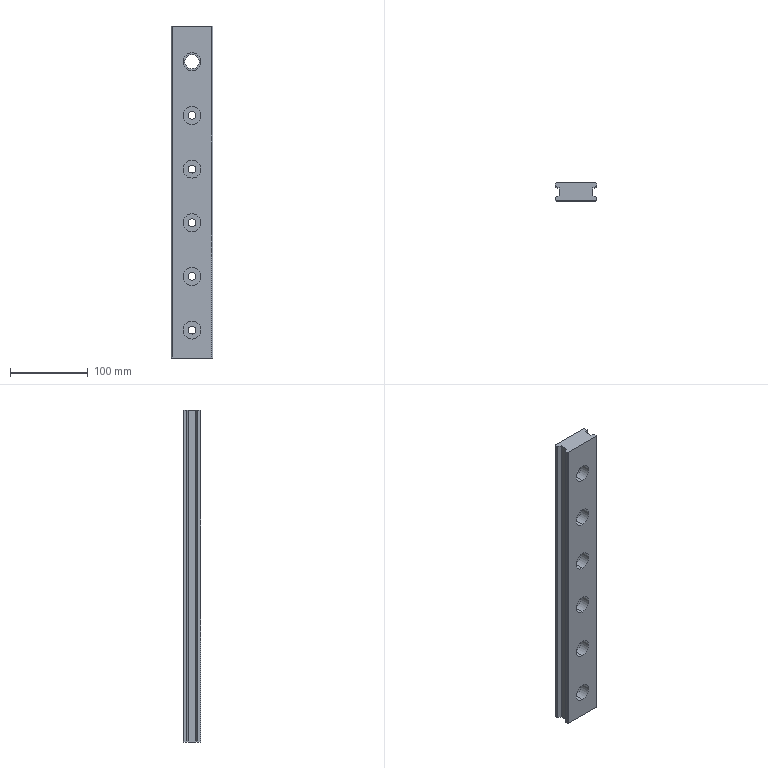Part | SolidWorks | features BaseBody 1 | 1 solid | 48 faces | box 53.538 x 23.077 x 428.351 mm | volume 438596 mm3 | cylinder 24 | plane 24 | commonest cylinder face diameters 23.077 x12 10.385 x10 18.462 x2
STEP:
#1=CARTESIAN_POINT('',(57.247,344.808,-35.962));
#2=VERTEX_POINT('',#1);
#3=CARTESIAN_POINT('',(57.247,344.808,-25.577));
#4=VERTEX_POINT('',#3);
#5=CARTESIAN_POINT('',(57.247,344.808,-30.769));
#6=DIRECTION('',(0.,1.,0.));
#7=DIRECTION('',(0.,0.,1.));
#8=AXIS2_PLACEMENT_3D('',#5,#6,#7);
#9=CIRCLE('',#8,5.192);
#10=EDGE_CURVE('',#2,#4,#9,.T.);
#11=ORIENTED_EDGE('',*,*,#10,.F.);
#12=CARTESIAN_POINT('',(57.247,354.5,-35.962));
#13=VERTEX_POINT('',#12);
#14=CARTESIAN_POINT('',(57.247,329.115,-35.962));
#15=DIRECTION('',(0.,1.,0.));
#16=VECTOR('',#15,1000.);
#17=LINE('',#14,#16);
#18=EDGE_CURVE('',#2,#13,#17,.T.);
#19=ORIENTED_EDGE('',*,*,#18,.T.);
#20=CARTESIAN_POINT('',(57.247,354.5,-25.577));
#21=VERTEX_POINT('',#20);
#22=CARTESIAN_POINT('',(57.247,354.5,-30.769));
#23=DIRECTION('',(0.,1.,0.));
#24=DIRECTION('',(0.,0.,1.));
#25=AXIS2_PLACEMENT_3D('',#22,#23,#24);
#26=CIRCLE('',#25,5.192);
#27=EDGE_CURVE('',#13,#21,#26,.T.);
#28=ORIENTED_EDGE('',*,*,#27,.T.);
#29=CARTESIAN_POINT('',(57.247,329.115,-25.577));
#30=DIRECTION('',(0.,1.,0.));
#31=VECTOR('',#30,1000.);
#32=LINE('',#29,#31);
#33=EDGE_CURVE('',#4,#21,#32,.T.);
#34=ORIENTED_EDGE('',*,*,#33,.F.);
#35=EDGE_LOOP('',(#11,#19,#28,#34));
#36=FACE_OUTER_BOUND('',#35,.T.);
#37=CARTESIAN_POINT('',(57.247,329.115,-30.769));
#38=DIRECTION('',(0.,1.,0.));
#39=DIRECTION('',(0.,0.,1.));
#40=AXIS2_PLACEMENT_3D('',#37,#38,#39);
#41=CYLINDRICAL_SURFACE('',#40,5.192);
#42=ADVANCED_FACE('',(#36),#41,.F.);
#43=CARTESIAN_POINT('',(57.247,344.808,102.5));
#44=VERTEX_POINT('',#43);
#45=CARTESIAN_POINT('',(57.247,344.808,112.885));
#46=VERTEX_POINT('',#45);
#47=CARTESIAN_POINT('',(57.247,344.808,107.692));
#48=DIRECTION('',(0.,1.,0.));
#49=DIRECTION('',(0.,0.,1.));
#50=AXIS2_PLACEMENT_3D('',#47,#48,#49);
#51=CIRCLE('',#50,5.192);
#52=EDGE_CURVE('',#44,#46,#51,.T.);
#53=ORIENTED_EDGE('',*,*,#52,.F.);
#54=CARTESIAN_POINT('',(57.247,354.5,102.5));
#55=VERTEX_POINT('',#54);
#56=CARTESIAN_POINT('',(57.247,329.115,102.5));
#57=DIRECTION('',(0.,1.,0.));
#58=VECTOR('',#57,1000.);
#59=LINE('',#56,#58);
#60=EDGE_CURVE('',#44,#55,#59,.T.);
#61=ORIENTED_EDGE('',*,*,#60,.T.);
#62=CARTESIAN_POINT('',(57.247,354.5,112.885));
#63=VERTEX_POINT('',#62);
#64=CARTESIAN_POINT('',(57.247,354.5,107.692));
#65=DIRECTION('',(0.,1.,0.));
#66=DIRECTION('',(0.,0.,1.));
#67=AXIS2_PLACEMENT_3D('',#64,#65,#66);
#68=CIRCLE('',#67,5.192);
#69=EDGE_CURVE('',#55,#63,#68,.T.);
#70=ORIENTED_EDGE('',*,*,#69,.T.);
#71=CARTESIAN_POINT('',(57.247,329.115,112.885));
#72=DIRECTION('',(0.,1.,0.));
#73=VECTOR('',#72,1000.);
#74=LINE('',#71,#73);
#75=EDGE_CURVE('',#46,#63,#74,.T.);
#76=ORIENTED_EDGE('',*,*,#75,.F.);
#77=EDGE_LOOP('',(#53,#61,#70,#76));
#78=FACE_OUTER_BOUND('',#77,.T.);
#79=CARTESIAN_POINT('',(57.247,329.115,107.692));
#80=DIRECTION('',(0.,1.,0.));
#81=DIRECTION('',(0.,0.,1.));
#82=AXIS2_PLACEMENT_3D('',#79,#80,#81);
#83=CYLINDRICAL_SURFACE('',#82,5.192);
#84=ADVANCED_FACE('',(#78),#83,.F.);
#85=CARTESIAN_POINT('',(57.247,344.808,236.923));
#86=VERTEX_POINT('',#85);
#87=CARTESIAN_POINT('',(57.247,344.808,255.385));
#88=VERTEX_POINT('',#87);
#89=CARTESIAN_POINT('',(57.247,344.808,246.154));
#90=DIRECTION('',(0.,1.,0.));
#91=DIRECTION('',(0.,0.,1.));
#92=AXIS2_PLACEMENT_3D('',#89,#90,#91);
#93=CIRCLE('',#92,9.231);
#94=EDGE_CURVE('',#86,#88,#93,.T.);
#95=ORIENTED_EDGE('',*,*,#94,.F.);
#96=CARTESIAN_POINT('',(57.247,354.5,236.923));
#97=VERTEX_POINT('',#96);
#98=CARTESIAN_POINT('',(57.247,329.115,236.923));
#99=DIRECTION('',(0.,1.,0.));
#100=VECTOR('',#99,1000.);
#101=LINE('',#98,#100);
#102=EDGE_CURVE('',#86,#97,#101,.T.);
#103=ORIENTED_EDGE('',*,*,#102,.T.);
#104=CARTESIAN_POINT('',(57.247,354.5,255.385));
#105=VERTEX_POINT('',#104);
#106=CARTESIAN_POINT('',(57.247,354.5,246.154));
#107=DIRECTION('',(0.,1.,0.));
#108=DIRECTION('',(0.,0.,1.));
#109=AXIS2_PLACEMENT_3D('',#106,#107,#108);
#110=CIRCLE('',#109,9.231);
#111=EDGE_CURVE('',#97,#105,#110,.T.);
#112=ORIENTED_EDGE('',*,*,#111,.T.);
#113=CARTESIAN_POINT('',(57.247,329.115,255.385));
#114=DIRECTION('',(0.,1.,0.));
#115=VECTOR('',#114,1000.);
#116=LINE('',#113,#115);
#117=EDGE_CURVE('',#88,#105,#116,.T.);
#118=ORIENTED_EDGE('',*,*,#117,.F.);
#119=EDGE_LOOP('',(#95,#103,#112,#118));
#120=FACE_OUTER_BOUND('',#119,.T.);
#121=CARTESIAN_POINT('',(57.247,329.115,246.154));
#122=DIRECTION('',(0.,1.,0.));
#123=DIRECTION('',(0.,0.,1.));
#124=AXIS2_PLACEMENT_3D('',#121,#122,#123);
#125=CYLINDRICAL_SURFACE('',#124,9.231);
#126=ADVANCED_FACE('',(#120),#125,.F.);
#127=CARTESIAN_POINT('',(57.247,344.808,-105.192));
#128=VERTEX_POINT('',#127);
#129=CARTESIAN_POINT('',(57.247,344.808,-94.808));
#130=VERTEX_POINT('',#129);
#131=CARTESIAN_POINT('',(57.247,344.808,-100.));
#132=DIRECTION('',(0.,1.,0.));
#133=DIRECTION('',(0.,0.,1.));
#134=AXIS2_PLACEMENT_3D('',#131,#132,#133);
#135=CIRCLE('',#134,5.192);
#136=EDGE_CURVE('',#128,#130,#135,.T.);
#137=ORIENTED_EDGE('',*,*,#136,.F.);
#138=CARTESIAN_POINT('',(57.247,354.5,-105.192));
#139=VERTEX_POINT('',#138);
#140=CARTESIAN_POINT('',(57.247,329.115,-105.192));
#141=DIRECTION('',(0.,1.,0.));
#142=VECTOR('',#141,1000.);
#143=LINE('',#140,#142);
#144=EDGE_CURVE('',#128,#139,#143,.T.);
#145=ORIENTED_EDGE('',*,*,#144,.T.);
#146=CARTESIAN_POINT('',(57.247,354.5,-94.808));
#147=VERTEX_POINT('',#146);
#148=CARTESIAN_POINT('',(57.247,354.5,-100.));
#149=DIRECTION('',(0.,1.,0.));
#150=DIRECTION('',(0.,0.,1.));
#151=AXIS2_PLACEMENT_3D('',#148,#149,#150);
#152=CIRCLE('',#151,5.192);
#153=EDGE_CURVE('',#139,#147,#152,.T.);
#154=ORIENTED_EDGE('',*,*,#153,.T.);
#155=CARTESIAN_POINT('',(57.247,329.115,-94.808));
#156=DIRECTION('',(0.,1.,0.));
#157=VECTOR('',#156,1000.);
#158=LINE('',#155,#157);
#159=EDGE_CURVE('',#130,#147,#158,.T.);
#160=ORIENTED_EDGE('',*,*,#159,.F.);
#161=EDGE_LOOP('',(#137,#145,#154,#160));
#162=FACE_OUTER_BOUND('',#161,.T.);
#163=CARTESIAN_POINT('',(57.247,329.115,-100.));
#164=DIRECTION('',(0.,1.,0.));
#165=DIRECTION('',(0.,0.,1.));
#166=AXIS2_PLACEMENT_3D('',#163,#164,#165);
#167=CYLINDRICAL_SURFACE('',#166,5.192);
#168=ADVANCED_FACE('',(#162),#167,.F.);
#169=CARTESIAN_POINT('',(57.247,344.808,171.731));
#170=VERTEX_POINT('',#169);
#171=CARTESIAN_POINT('',(57.247,344.808,182.115));
#172=VERTEX_POINT('',#171);
#173=CARTESIAN_POINT('',(57.247,344.808,176.923));
#174=DIRECTION('',(0.,1.,0.));
#175=DIRECTION('',(0.,0.,1.));
#176=AXIS2_PLACEMENT_3D('',#173,#174,#175);
#177=CIRCLE('',#176,5.192);
#178=EDGE_CURVE('',#170,#172,#177,.T.);
#179=ORIENTED_EDGE('',*,*,#178,.F.);
#180=CARTESIAN_POINT('',(57.247,354.5,171.731));
#181=VERTEX_POINT('',#180);
#182=CARTESIAN_POINT('',(57.247,329.115,171.731));
#183=DIRECTION('',(0.,1.,0.));
#184=VECTOR('',#183,1000.);
#185=LINE('',#182,#184);
#186=EDGE_CURVE('',#170,#181,#185,.T.);
#187=ORIENTED_EDGE('',*,*,#186,.T.);
#188=CARTESIAN_POINT('',(57.247,354.5,182.115));
#189=VERTEX_POINT('',#188);
#190=CARTESIAN_POINT('',(57.247,354.5,176.923));
#191=DIRECTION('',(0.,1.,0.));
#192=DIRECTION('',(0.,0.,1.));
#193=AXIS2_PLACEMENT_3D('',#190,#191,#192);
#194=CIRCLE('',#193,5.192);
#195=EDGE_CURVE('',#181,#189,#194,.T.);
#196=ORIENTED_EDGE('',*,*,#195,.T.);
#197=CARTESIAN_POINT('',(57.247,329.115,182.115));
#198=DIRECTION('',(0.,1.,0.));
#199=VECTOR('',#198,1000.);
#200=LINE('',#197,#199);
#201=EDGE_CURVE('',#172,#189,#200,.T.);
#202=ORIENTED_EDGE('',*,*,#201,.F.);
#203=EDGE_LOOP('',(#179,#187,#196,#202));
#204=FACE_OUTER_BOUND('',#203,.T.);
#205=CARTESIAN_POINT('',(57.247,329.115,176.923));
#206=DIRECTION('',(0.,1.,0.));
#207=DIRECTION('',(0.,0.,1.));
#208=AXIS2_PLACEMENT_3D('',#205,#206,#207);
#209=CYLINDRICAL_SURFACE('',#208,5.192);
#210=ADVANCED_FACE('',(#204),#209,.F.);
#211=CARTESIAN_POINT('',(57.247,344.808,33.269));
#212=VERTEX_POINT('',#211);
#213=CARTESIAN_POINT('',(57.247,344.808,43.654));
#214=VERTEX_POINT('',#213);
#215=CARTESIAN_POINT('',(57.247,344.808,38.462));
#216=DIRECTION('',(0.,1.,0.));
#217=DIRECTION('',(0.,0.,1.));
#218=AXIS2_PLACEMENT_3D('',#215,#216,#217);
#219=CIRCLE('',#218,5.192);
#220=EDGE_CURVE('',#212,#214,#219,.T.);
#221=ORIENTED_EDGE('',*,*,#220,.F.);
#222=CARTESIAN_POINT('',(57.247,354.5,33.269));
#223=VERTEX_POINT('',#222);
#224=CARTESIAN_POINT('',(57.247,329.115,33.269));
#225=DIRECTION('',(0.,1.,0.));
#226=VECTOR('',#225,1000.);
#227=LINE('',#224,#226);
#228=EDGE_CURVE('',#212,#223,#227,.T.);
#229=ORIENTED_EDGE('',*,*,#228,.T.);
#230=CARTESIAN_POINT('',(57.247,354.5,43.654));
#231=VERTEX_POINT('',#230);
#232=CARTESIAN_POINT('',(57.247,354.5,38.462));
#233=DIRECTION('',(0.,1.,0.));
#234=DIRECTION('',(0.,0.,1.));
#235=AXIS2_PLACEMENT_3D('',#232,#233,#234);
#236=CIRCLE('',#235,5.192);
#237=EDGE_CURVE('',#223,#231,#236,.T.);
#238=ORIENTED_EDGE('',*,*,#237,.T.);
#239=CARTESIAN_POINT('',(57.247,329.115,43.654));
#240=DIRECTION('',(0.,1.,0.));
#241=VECTOR('',#240,1000.);
#242=LINE('',#239,#241);
#243=EDGE_CURVE('',#214,#231,#242,.T.);
#244=ORIENTED_EDGE('',*,*,#243,.F.);
#245=EDGE_LOOP('',(#221,#229,#238,#244));
#246=FACE_OUTER_BOUND('',#245,.T.);
#247=CARTESIAN_POINT('',(57.247,329.115,38.462));
#248=DIRECTION('',(0.,1.,0.));
#249=DIRECTION('',(0.,0.,1.));
#250=AXIS2_PLACEMENT_3D('',#247,#248,#249);
#251=CYLINDRICAL_SURFACE('',#250,5.192);
#252=ADVANCED_FACE('',(#246),#251,.F.);
#253=CARTESIAN_POINT('',(57.247,331.423,-19.231));
#254=VERTEX_POINT('',#253);
#255=CARTESIAN_POINT('',(57.247,331.423,-42.308));
#256=VERTEX_POINT('',#255);
#257=CARTESIAN_POINT('',(57.247,331.423,-30.769));
#258=DIRECTION('',(0.,-1.,0.));
#259=DIRECTION('',(0.,0.,1.));
#260=AXIS2_PLACEMENT_3D('',#257,#258,#259);
#261=CIRCLE('',#260,11.538);
#262=EDGE_CURVE('',#254,#256,#261,.T.);
#263=ORIENTED_EDGE('',*,*,#262,.T.);
#264=CARTESIAN_POINT('',(57.247,344.808,-42.308));
#265=VERTEX_POINT('',#264);
#266=CARTESIAN_POINT('',(57.247,329.115,-42.308));
#267=DIRECTION('',(0.,1.,0.));
#268=VECTOR('',#267,1000.);
#269=LINE('',#266,#268);
#270=EDGE_CURVE('',#256,#265,#269,.T.);
#271=ORIENTED_EDGE('',*,*,#270,.T.);
#272=CARTESIAN_POINT('',(57.247,344.808,-19.231));
#273=VERTEX_POINT('',#272);
#274=CARTESIAN_POINT('',(57.247,344.808,-30.769));
#275=DIRECTION('',(0.,-1.,0.));
#276=DIRECTION('',(0.,0.,1.));
#277=AXIS2_PLACEMENT_3D('',#274,#275,#276);
#278=CIRCLE('',#277,11.538);
#279=EDGE_CURVE('',#273,#265,#278,.T.);
#280=ORIENTED_EDGE('',*,*,#279,.F.);
#281=CARTESIAN_POINT('',(57.247,329.115,-19.231));
#282=DIRECTION('',(0.,1.,0.));
#283=VECTOR('',#282,1000.);
#284=LINE('',#281,#283);
#285=EDGE_CURVE('',#254,#273,#284,.T.);
#286=ORIENTED_EDGE('',*,*,#285,.F.);
#287=EDGE_LOOP('',(#263,#271,#280,#286));
#288=FACE_OUTER_BOUND('',#287,.T.);
#289=CARTESIAN_POINT('',(57.247,329.115,-30.769));
#290=DIRECTION('',(0.,1.,0.));
#291=DIRECTION('',(0.,0.,1.));
#292=AXIS2_PLACEMENT_3D('',#289,#290,#291);
#293=CYLINDRICAL_SURFACE('',#292,11.538);
#294=ADVANCED_FACE('',(#288),#293,.F.);
#295=CARTESIAN_POINT('',(57.247,331.423,119.231));
#296=VERTEX_POINT('',#295);
#297=CARTESIAN_POINT('',(57.247,331.423,96.154));
#298=VERTEX_POINT('',#297);
#299=CARTESIAN_POINT('',(57.247,331.423,107.692));
#300=DIRECTION('',(0.,-1.,0.));
#301=DIRECTION('',(0.,0.,1.));
#302=AXIS2_PLACEMENT_3D('',#299,#300,#301);
#303=CIRCLE('',#302,11.538);
#304=EDGE_CURVE('',#296,#298,#303,.T.);
#305=ORIENTED_EDGE('',*,*,#304,.T.);
#306=CARTESIAN_POINT('',(57.247,344.808,96.154));
#307=VERTEX_POINT('',#306);
#308=CARTESIAN_POINT('',(57.247,329.115,96.154));
#309=DIRECTION('',(0.,1.,0.));
#310=VECTOR('',#309,1000.);
#311=LINE('',#308,#310);
#312=EDGE_CURVE('',#298,#307,#311,.T.);
#313=ORIENTED_EDGE('',*,*,#312,.T.);
#314=CARTESIAN_POINT('',(57.247,344.808,119.231));
#315=VERTEX_POINT('',#314);
#316=CARTESIAN_POINT('',(57.247,344.808,107.692));
#317=DIRECTION('',(0.,-1.,0.));
#318=DIRECTION('',(0.,0.,1.));
#319=AXIS2_PLACEMENT_3D('',#316,#317,#318);
#320=CIRCLE('',#319,11.538);
#321=EDGE_CURVE('',#315,#307,#320,.T.);
#322=ORIENTED_EDGE('',*,*,#321,.F.);
#323=CARTESIAN_POINT('',(57.247,329.115,119.231));
#324=DIRECTION('',(0.,1.,0.));
#325=VECTOR('',#324,1000.);
#326=LINE('',#323,#325);
#327=EDGE_CURVE('',#296,#315,#326,.T.);
#328=ORIENTED_EDGE('',*,*,#327,.F.);
#329=EDGE_LOOP('',(#305,#313,#322,#328));
#330=FACE_OUTER_BOUND('',#329,.T.);
#331=CARTESIAN_POINT('',(57.247,329.115,107.692));
#332=DIRECTION('',(0.,1.,0.));
#333=DIRECTION('',(0.,0.,1.));
#334=AXIS2_PLACEMENT_3D('',#331,#332,#333);
#335=CYLINDRICAL_SURFACE('',#334,11.538);
#336=ADVANCED_FACE('',(#330),#335,.F.);
#337=CARTESIAN_POINT('',(57.247,331.423,257.692));
#338=VERTEX_POINT('',#337);
#339=CARTESIAN_POINT('',(57.247,331.423,234.615));
#340=VERTEX_POINT('',#339);
#341=CARTESIAN_POINT('',(57.247,331.423,246.154));
#342=DIRECTION('',(0.,-1.,0.));
#343=DIRECTION('',(0.,0.,1.));
#344=AXIS2_PLACEMENT_3D('',#341,#342,#343);
#345=CIRCLE('',#344,11.538);
#346=EDGE_CURVE('',#338,#340,#345,.T.);
#347=ORIENTED_EDGE('',*,*,#346,.T.);
#348=CARTESIAN_POINT('',(57.247,344.808,234.615));
#349=VERTEX_POINT('',#348);
#350=CARTESIAN_POINT('',(57.247,329.115,234.615));
#351=DIRECTION('',(0.,1.,0.));
#352=VECTOR('',#351,1000.);
#353=LINE('',#350,#352);
#354=EDGE_CURVE('',#340,#349,#353,.T.);
#355=ORIENTED_EDGE('',*,*,#354,.T.);
#356=CARTESIAN_POINT('',(57.247,344.808,257.692));
#357=VERTEX_POINT('',#356);
#358=CARTESIAN_POINT('',(57.247,344.808,246.154));
#359=DIRECTION('',(0.,-1.,0.));
#360=DIRECTION('',(0.,0.,1.));
#361=AXIS2_PLACEMENT_3D('',#358,#359,#360);
#362=CIRCLE('',#361,11.538);
#363=EDGE_CURVE('',#357,#349,#362,.T.);
#364=ORIENTED_EDGE('',*,*,#363,.F.);
#365=CARTESIAN_POINT('',(57.247,329.115,257.692));
#366=DIRECTION('',(0.,1.,0.));
#367=VECTOR('',#366,1000.);
#368=LINE('',#365,#367);
#369=EDGE_CURVE('',#338,#357,#368,.T.);
#370=ORIENTED_EDGE('',*,*,#369,.F.);
#371=EDGE_LOOP('',(#347,#355,#364,#370));
#372=FACE_OUTER_BOUND('',#371,.T.);
#373=CARTESIAN_POINT('',(57.247,329.115,246.154));
#374=DIRECTION('',(0.,1.,0.));
#375=DIRECTION('',(0.,0.,1.));
#376=AXIS2_PLACEMENT_3D('',#373,#374,#375);
#377=CYLINDRICAL_SURFACE('',#376,11.538);
#378=ADVANCED_FACE('',(#372),#377,.F.);
#379=CARTESIAN_POINT('',(57.247,331.423,-88.462));
#380=VERTEX_POINT('',#379);
#381=CARTESIAN_POINT('',(57.247,331.423,-111.538));
#382=VERTEX_POINT('',#381);
#383=CARTESIAN_POINT('',(57.247,331.423,-100.));
#384=DIRECTION('',(0.,-1.,0.));
#385=DIRECTION('',(0.,0.,1.));
#386=AXIS2_PLACEMENT_3D('',#383,#384,#385);
#387=CIRCLE('',#386,11.538);
#388=EDGE_CURVE('',#380,#382,#387,.T.);
#389=ORIENTED_EDGE('',*,*,#388,.T.);
#390=CARTESIAN_POINT('',(57.247,344.808,-111.538));
#391=VERTEX_POINT('',#390);
#392=CARTESIAN_POINT('',(57.247,329.115,-111.538));
#393=DIRECTION('',(0.,1.,0.));
#394=VECTOR('',#393,1000.);
#395=LINE('',#392,#394);
#396=EDGE_CURVE('',#382,#391,#395,.T.);
#397=ORIENTED_EDGE('',*,*,#396,.T.);
#398=CARTESIAN_POINT('',(57.247,344.808,-88.462));
#399=VERTEX_POINT('',#398);
#400=CARTESIAN_POINT('',(57.247,344.808,-100.));
#401=DIRECTION('',(0.,-1.,0.));
#402=DIRECTION('',(0.,0.,1.));
#403=AXIS2_PLACEMENT_3D('',#400,#401,#402);
#404=CIRCLE('',#403,11.538);
#405=EDGE_CURVE('',#399,#391,#404,.T.);
#406=ORIENTED_EDGE('',*,*,#405,.F.);
#407=CARTESIAN_POINT('',(57.247,329.115,-88.462));
#408=DIRECTION('',(0.,1.,0.));
#409=VECTOR('',#408,1000.);
#410=LINE('',#407,#409);
#411=EDGE_CURVE('',#380,#399,#410,.T.);
#412=ORIENTED_EDGE('',*,*,#411,.F.);
#413=EDGE_LOOP('',(#389,#397,#406,#412));
#414=FACE_OUTER_BOUND('',#413,.T.);
#415=CARTESIAN_POINT('',(57.247,329.115,-100.));
#416=DIRECTION('',(0.,1.,0.));
#417=DIRECTION('',(0.,0.,1.));
#418=AXIS2_PLACEMENT_3D('',#415,#416,#417);
#419=CYLINDRICAL_SURFACE('',#418,11.538);
#420=ADVANCED_FACE('',(#414),#419,.F.);
#421=CARTESIAN_POINT('',(57.247,331.423,188.462));
#422=VERTEX_POINT('',#421);
#423=CARTESIAN_POINT('',(57.247,331.423,165.385));
#424=VERTEX_POINT('',#423);
#425=CARTESIAN_POINT('',(57.247,331.423,176.923));
#426=DIRECTION('',(0.,-1.,0.));
#427=DIRECTION('',(0.,0.,1.));
#428=AXIS2_PLACEMENT_3D('',#425,#426,#427);
#429=CIRCLE('',#428,11.538);
#430=EDGE_CURVE('',#422,#424,#429,.T.);
#431=ORIENTED_EDGE('',*,*,#430,.T.);
#432=CARTESIAN_POINT('',(57.247,344.808,165.385));
#433=VERTEX_POINT('',#432);
#434=CARTESIAN_POINT('',(57.247,329.115,165.385));
#435=DIRECTION('',(0.,1.,0.));
#436=VECTOR('',#435,1000.);
#437=LINE('',#434,#436);
#438=EDGE_CURVE('',#424,#433,#437,.T.);
#439=ORIENTED_EDGE('',*,*,#438,.T.);
#440=CARTESIAN_POINT('',(57.247,344.808,188.462));
#441=VERTEX_POINT('',#440);
#442=CARTESIAN_POINT('',(57.247,344.808,176.923));
#443=DIRECTION('',(0.,-1.,0.));
#444=DIRECTION('',(0.,0.,1.));
#445=AXIS2_PLACEMENT_3D('',#442,#443,#444);
#446=CIRCLE('',#445,11.538);
#447=EDGE_CURVE('',#441,#433,#446,.T.);
#448=ORIENTED_EDGE('',*,*,#447,.F.);
#449=CARTESIAN_POINT('',(57.247,329.115,188.462));
#450=DIRECTION('',(0.,1.,0.));
#451=VECTOR('',#450,1000.);
#452=LINE('',#449,#451);
#453=EDGE_CURVE('',#422,#441,#452,.T.);
#454=ORIENTED_EDGE('',*,*,#453,.F.);
#455=EDGE_LOOP('',(#431,#439,#448,#454));
#456=FACE_OUTER_BOUND('',#455,.T.);
#457=CARTESIAN_POINT('',(57.247,329.115,176.923));
#458=DIRECTION('',(0.,1.,0.));
#459=DIRECTION('',(0.,0.,1.));
#460=AXIS2_PLACEMENT_3D('',#457,#458,#459);
#461=CYLINDRICAL_SURFACE('',#460,11.538);
#462=ADVANCED_FACE('',(#456),#461,.F.);
#463=CARTESIAN_POINT('',(57.247,331.423,50.));
#464=VERTEX_POINT('',#463);
#465=CARTESIAN_POINT('',(57.247,331.423,26.923));
#466=VERTEX_POINT('',#465);
#467=CARTESIAN_POINT('',(57.247,331.423,38.462));
#468=DIRECTION('',(0.,-1.,0.));
#469=DIRECTION('',(0.,0.,1.));
#470=AXIS2_PLACEMENT_3D('',#467,#468,#469);
#471=CIRCLE('',#470,11.538);
#472=EDGE_CURVE('',#464,#466,#471,.T.);
#473=ORIENTED_EDGE('',*,*,#472,.T.);
#474=CARTESIAN_POINT('',(57.247,344.808,26.923));
#475=VERTEX_POINT('',#474);
#476=CARTESIAN_POINT('',(57.247,329.115,26.923));
#477=DIRECTION('',(0.,1.,0.));
#478=VECTOR('',#477,1000.);
#479=LINE('',#476,#478);
#480=EDGE_CURVE('',#466,#475,#479,.T.);
#481=ORIENTED_EDGE('',*,*,#480,.T.);
#482=CARTESIAN_POINT('',(57.247,344.808,50.));
#483=VERTEX_POINT('',#482);
#484=CARTESIAN_POINT('',(57.247,344.808,38.462));
#485=DIRECTION('',(0.,-1.,0.));
#486=DIRECTION('',(0.,0.,1.));
#487=AXIS2_PLACEMENT_3D('',#484,#485,#486);
#488=CIRCLE('',#487,11.538);
#489=EDGE_CURVE('',#483,#475,#488,.T.);
#490=ORIENTED_EDGE('',*,*,#489,.F.);
#491=CARTESIAN_POINT('',(57.247,329.115,50.));
#492=DIRECTION('',(0.,1.,0.));
#493=VECTOR('',#492,1000.);
#494=LINE('',#491,#493);
#495=EDGE_CURVE('',#464,#483,#494,.T.);
#496=ORIENTED_EDGE('',*,*,#495,.F.);
#497=EDGE_LOOP('',(#473,#481,#490,#496));
#498=FACE_OUTER_BOUND('',#497,.T.);
#499=CARTESIAN_POINT('',(57.247,329.115,38.462));
#500=DIRECTION('',(0.,1.,0.));
#501=DIRECTION('',(0.,0.,1.));
#502=AXIS2_PLACEMENT_3D('',#499,#500,#501);
#503=CYLINDRICAL_SURFACE('',#502,11.538);
#504=ADVANCED_FACE('',(#498),#503,.F.);
#505=CARTESIAN_POINT('',(57.247,354.5,-30.769));
#506=DIRECTION('',(0.,1.,0.));
#507=DIRECTION('',(0.,0.,1.));
#508=AXIS2_PLACEMENT_3D('',#505,#506,#507);
#509=CIRCLE('',#508,5.192);
#510=EDGE_CURVE('',#21,#13,#509,.T.);
#511=ORIENTED_EDGE('',*,*,#510,.F.);
#512=ORIENTED_EDGE('',*,*,#27,.F.);
#513=EDGE_LOOP('',(#511,#512));
#514=FACE_BOUND('',#513,.T.);
#515=CARTESIAN_POINT('',(57.247,354.5,107.692));
#516=DIRECTION('',(0.,1.,0.));
#517=DIRECTION('',(0.,0.,1.));
#518=AXIS2_PLACEMENT_3D('',#515,#516,#517);
#519=CIRCLE('',#518,5.192);
#520=EDGE_CURVE('',#63,#55,#519,.T.);
#521=ORIENTED_EDGE('',*,*,#520,.F.);
#522=ORIENTED_EDGE('',*,*,#69,.F.);
#523=EDGE_LOOP('',(#521,#522));
#524=FACE_BOUND('',#523,.T.);
#525=CARTESIAN_POINT('',(57.247,354.5,246.154));
#526=DIRECTION('',(0.,1.,0.));
#527=DIRECTION('',(0.,0.,1.));
#528=AXIS2_PLACEMENT_3D('',#525,#526,#527);
#529=CIRCLE('',#528,9.231);
#530=EDGE_CURVE('',#105,#97,#529,.T.);
#531=ORIENTED_EDGE('',*,*,#530,.F.);
#532=ORIENTED_EDGE('',*,*,#111,.F.);
#533=EDGE_LOOP('',(#531,#532));
#534=FACE_BOUND('',#533,.T.);
#535=CARTESIAN_POINT('',(57.247,354.5,-100.));
#536=DIRECTION('',(0.,1.,0.));
#537=DIRECTION('',(0.,0.,1.));
#538=AXIS2_PLACEMENT_3D('',#535,#536,#537);
#539=CIRCLE('',#538,5.192);
#540=EDGE_CURVE('',#147,#139,#539,.T.);
#541=ORIENTED_EDGE('',*,*,#540,.F.);
#542=ORIENTED_EDGE('',*,*,#153,.F.);
#543=EDGE_LOOP('',(#541,#542));
#544=FACE_BOUND('',#543,.T.);
#545=CARTESIAN_POINT('',(57.247,354.5,176.923));
#546=DIRECTION('',(0.,1.,0.));
#547=DIRECTION('',(0.,0.,1.));
#548=AXIS2_PLACEMENT_3D('',#545,#546,#547);
#549=CIRCLE('',#548,5.192);
#550=EDGE_CURVE('',#189,#181,#549,.T.);
#551=ORIENTED_EDGE('',*,*,#550,.F.);
#552=ORIENTED_EDGE('',*,*,#195,.F.);
#553=EDGE_LOOP('',(#551,#552));
#554=FACE_BOUND('',#553,.T.);
#555=CARTESIAN_POINT('',(57.247,354.5,38.462));
#556=DIRECTION('',(0.,1.,0.));
#557=DIRECTION('',(0.,0.,1.));
#558=AXIS2_PLACEMENT_3D('',#555,#556,#557);
#559=CIRCLE('',#558,5.192);
#560=EDGE_CURVE('',#231,#223,#559,.T.);
#561=ORIENTED_EDGE('',*,*,#560,.F.);
#562=ORIENTED_EDGE('',*,*,#237,.F.);
#563=EDGE_LOOP('',(#561,#562));
#564=FACE_BOUND('',#563,.T.);
#565=CARTESIAN_POINT('',(31.631,354.5,292.308));
#566=VERTEX_POINT('',#565);
#567=CARTESIAN_POINT('',(31.631,354.5,-136.043));
#568=VERTEX_POINT('',#567);
#569=CARTESIAN_POINT('',(31.631,354.5,-284.615));
#570=DIRECTION('',(0.,0.,-1.));
#571=VECTOR('',#570,1000.);
#572=LINE('',#569,#571);
#573=EDGE_CURVE('',#566,#568,#572,.T.);
#574=ORIENTED_EDGE('',*,*,#573,.F.);
#575=CARTESIAN_POINT('',(82.862,354.5,292.308));
#576=VERTEX_POINT('',#575);
#577=CARTESIAN_POINT('',(31.631,354.5,292.308));
#578=DIRECTION('',(-1.,0.,0.));
#579=VECTOR('',#578,1000.);
#580=LINE('',#577,#579);
#581=EDGE_CURVE('',#576,#566,#580,.T.);
#582=ORIENTED_EDGE('',*,*,#581,.F.);
#583=CARTESIAN_POINT('',(82.862,354.5,-136.043));
#584=VERTEX_POINT('',#583);
#585=CARTESIAN_POINT('',(82.862,354.5,-284.615));
#586=DIRECTION('',(0.,0.,1.));
#587=VECTOR('',#586,1000.);
#588=LINE('',#585,#587);
#589=EDGE_CURVE('',#584,#576,#588,.T.);
#590=ORIENTED_EDGE('',*,*,#589,.F.);
#591=CARTESIAN_POINT('',(31.631,354.5,-136.043));
#592=DIRECTION('',(1.,0.,0.));
#593=VECTOR('',#592,1000.);
#594=LINE('',#591,#593);
#595=EDGE_CURVE('',#568,#584,#594,.T.);
#596=ORIENTED_EDGE('',*,*,#595,.F.);
#597=EDGE_LOOP('',(#574,#582,#590,#596));
#598=FACE_OUTER_BOUND('',#597,.T.);
#599=CARTESIAN_POINT('',(31.631,354.5,-284.615));
#600=DIRECTION('',(0.,-1.,0.));
#601=DIRECTION('',(0.,0.,-1.));
#602=AXIS2_PLACEMENT_3D('',#599,#600,#601);
#603=PLANE('',#602);
#604=ADVANCED_FACE('',(#514,#524,#534,#544,#554,#564,#598),#603,.F.);
#605=ORIENTED_EDGE('',*,*,#18,.F.);
#606=CARTESIAN_POINT('',(57.247,344.808,-30.769));
#607=DIRECTION('',(0.,1.,0.));
#608=DIRECTION('',(0.,0.,1.));
#609=AXIS2_PLACEMENT_3D('',#606,#607,#608);
#610=CIRCLE('',#609,5.192);
#611=EDGE_CURVE('',#4,#2,#610,.T.);
#612=ORIENTED_EDGE('',*,*,#611,.F.);
#613=ORIENTED_EDGE('',*,*,#33,.T.);
#614=ORIENTED_EDGE('',*,*,#510,.T.);
#615=EDGE_LOOP('',(#605,#612,#613,#614));
#616=FACE_OUTER_BOUND('',#615,.T.);
#617=CARTESIAN_POINT('',(57.247,329.115,-30.769));
#618=DIRECTION('',(0.,1.,0.));
#619=DIRECTION('',(0.,0.,1.));
#620=AXIS2_PLACEMENT_3D('',#617,#618,#619);
#621=CYLINDRICAL_SURFACE('',#620,5.192);
#622=ADVANCED_FACE('',(#616),#621,.F.);
#623=ORIENTED_EDGE('',*,*,#60,.F.);
#624=CARTESIAN_POINT('',(57.247,344.808,107.692));
#625=DIRECTION('',(0.,1.,0.));
#626=DIRECTION('',(0.,0.,1.));
#627=AXIS2_PLACEMENT_3D('',#624,#625,#626);
#628=CIRCLE('',#627,5.192);
#629=EDGE_CURVE('',#46,#44,#628,.T.);
#630=ORIENTED_EDGE('',*,*,#629,.F.);
#631=ORIENTED_EDGE('',*,*,#75,.T.);
#632=ORIENTED_EDGE('',*,*,#520,.T.);
#633=EDGE_LOOP('',(#623,#630,#631,#632));
#634=FACE_OUTER_BOUND('',#633,.T.);
#635=CARTESIAN_POINT('',(57.247,329.115,107.692));
#636=DIRECTION('',(0.,1.,0.));
#637=DIRECTION('',(0.,0.,1.));
#638=AXIS2_PLACEMENT_3D('',#635,#636,#637);
#639=CYLINDRICAL_SURFACE('',#638,5.192);
#640=ADVANCED_FACE('',(#634),#639,.F.);
#641=ORIENTED_EDGE('',*,*,#102,.F.);
#642=CARTESIAN_POINT('',(57.247,344.808,246.154));
#643=DIRECTION('',(0.,1.,0.));
#644=DIRECTION('',(0.,0.,1.));
#645=AXIS2_PLACEMENT_3D('',#642,#643,#644);
#646=CIRCLE('',#645,9.231);
#647=EDGE_CURVE('',#88,#86,#646,.T.);
#648=ORIENTED_EDGE('',*,*,#647,.F.);
#649=ORIENTED_EDGE('',*,*,#117,.T.);
#650=ORIENTED_EDGE('',*,*,#530,.T.);
#651=EDGE_LOOP('',(#641,#648,#649,#650));
#652=FACE_OUTER_BOUND('',#651,.T.);
#653=CARTESIAN_POINT('',(57.247,329.115,246.154));
#654=DIRECTION('',(0.,1.,0.));
#655=DIRECTION('',(0.,0.,1.));
#656=AXIS2_PLACEMENT_3D('',#653,#654,#655);
#657=CYLINDRICAL_SURFACE('',#656,9.231);
#658=ADVANCED_FACE('',(#652),#657,.F.);
#659=ORIENTED_EDGE('',*,*,#144,.F.);
#660=CARTESIAN_POINT('',(57.247,344.808,-100.));
#661=DIRECTION('',(0.,1.,0.));
#662=DIRECTION('',(0.,0.,1.));
#663=AXIS2_PLACEMENT_3D('',#660,#661,#662);
#664=CIRCLE('',#663,5.192);
#665=EDGE_CURVE('',#130,#128,#664,.T.);
#666=ORIENTED_EDGE('',*,*,#665,.F.);
#667=ORIENTED_EDGE('',*,*,#159,.T.);
#668=ORIENTED_EDGE('',*,*,#540,.T.);
#669=EDGE_LOOP('',(#659,#666,#667,#668));
#670=FACE_OUTER_BOUND('',#669,.T.);
#671=CARTESIAN_POINT('',(57.247,329.115,-100.));
#672=DIRECTION('',(0.,1.,0.));
#673=DIRECTION('',(0.,0.,1.));
#674=AXIS2_PLACEMENT_3D('',#671,#672,#673);
#675=CYLINDRICAL_SURFACE('',#674,5.192);
#676=ADVANCED_FACE('',(#670),#675,.F.);
#677=ORIENTED_EDGE('',*,*,#186,.F.);
#678=CARTESIAN_POINT('',(57.247,344.808,176.923));
#679=DIRECTION('',(0.,1.,0.));
#680=DIRECTION('',(0.,0.,1.));
#681=AXIS2_PLACEMENT_3D('',#678,#679,#680);
#682=CIRCLE('',#681,5.192);
#683=EDGE_CURVE('',#172,#170,#682,.T.);
#684=ORIENTED_EDGE('',*,*,#683,.F.);
#685=ORIENTED_EDGE('',*,*,#201,.T.);
#686=ORIENTED_EDGE('',*,*,#550,.T.);
#687=EDGE_LOOP('',(#677,#684,#685,#686));
#688=FACE_OUTER_BOUND('',#687,.T.);
#689=CARTESIAN_POINT('',(57.247,329.115,176.923));
#690=DIRECTION('',(0.,1.,0.));
#691=DIRECTION('',(0.,0.,1.));
#692=AXIS2_PLACEMENT_3D('',#689,#690,#691);
#693=CYLINDRICAL_SURFACE('',#692,5.192);
#694=ADVANCED_FACE('',(#688),#693,.F.);
#695=ORIENTED_EDGE('',*,*,#228,.F.);
#696=CARTESIAN_POINT('',(57.247,344.808,38.462));
#697=DIRECTION('',(0.,1.,0.));
#698=DIRECTION('',(0.,0.,1.));
#699=AXIS2_PLACEMENT_3D('',#696,#697,#698);
#700=CIRCLE('',#699,5.192);
#701=EDGE_CURVE('',#214,#212,#700,.T.);
#702=ORIENTED_EDGE('',*,*,#701,.F.);
#703=ORIENTED_EDGE('',*,*,#243,.T.);
#704=ORIENTED_EDGE('',*,*,#560,.T.);
#705=EDGE_LOOP('',(#695,#702,#703,#704));
#706=FACE_OUTER_BOUND('',#705,.T.);
#707=CARTESIAN_POINT('',(57.247,329.115,38.462));
#708=DIRECTION('',(0.,1.,0.));
#709=DIRECTION('',(0.,0.,1.));
#710=AXIS2_PLACEMENT_3D('',#707,#708,#709);
#711=CYLINDRICAL_SURFACE('',#710,5.192);
#712=ADVANCED_FACE('',(#706),#711,.F.);
#713=CARTESIAN_POINT('',(84.016,353.346,-136.043));
#714=VERTEX_POINT('',#713);
#715=CARTESIAN_POINT('',(84.016,353.346,-136.043));
#716=DIRECTION('',(-0.7071,0.7071,0.));
#717=VECTOR('',#716,1000.);
#718=LINE('',#715,#717);
#719=EDGE_CURVE('',#714,#584,#718,.T.);
#720=ORIENTED_EDGE('',*,*,#719,.F.);
#721=CARTESIAN_POINT('',(84.016,349.654,-136.043));
#722=VERTEX_POINT('',#721);
#723=CARTESIAN_POINT('',(84.016,357.,-136.043));
#724=DIRECTION('',(0.,1.,0.));
#725=VECTOR('',#724,1000.);
#726=LINE('',#723,#725);
#727=EDGE_CURVE('',#722,#714,#726,.T.);
#728=ORIENTED_EDGE('',*,*,#727,.F.);
#729=CARTESIAN_POINT('',(79.17,347.89,-136.043));
#730=VERTEX_POINT('',#729);
#731=CARTESIAN_POINT('',(79.17,347.89,-136.043));
#732=DIRECTION('',(0.9397,0.342,0.));
#733=VECTOR('',#732,1000.);
#734=LINE('',#731,#733);
#735=EDGE_CURVE('',#730,#722,#734,.T.);
#736=ORIENTED_EDGE('',*,*,#735,.F.);
#737=CARTESIAN_POINT('',(79.17,337.802,-136.043));
#738=VERTEX_POINT('',#737);
#739=CARTESIAN_POINT('',(79.17,357.,-136.043));
#740=DIRECTION('',(0.,1.,0.));
#741=VECTOR('',#740,1000.);
#742=LINE('',#739,#741);
#743=EDGE_CURVE('',#738,#730,#742,.T.);
#744=ORIENTED_EDGE('',*,*,#743,.F.);
#745=CARTESIAN_POINT('',(84.016,336.038,-136.043));
#746=VERTEX_POINT('',#745);
#747=CARTESIAN_POINT('',(84.016,336.038,-136.043));
#748=DIRECTION('',(-0.9397,0.342,0.));
#749=VECTOR('',#748,1000.);
#750=LINE('',#747,#749);
#751=EDGE_CURVE('',#746,#738,#750,.T.);
#752=ORIENTED_EDGE('',*,*,#751,.F.);
#753=CARTESIAN_POINT('',(84.016,332.577,-136.043));
#754=VERTEX_POINT('',#753);
#755=CARTESIAN_POINT('',(84.016,357.,-136.043));
#756=DIRECTION('',(0.,1.,0.));
#757=VECTOR('',#756,1000.);
#758=LINE('',#755,#757);
#759=EDGE_CURVE('',#754,#746,#758,.T.);
#760=ORIENTED_EDGE('',*,*,#759,.F.);
#761=CARTESIAN_POINT('',(82.862,331.423,-136.043));
#762=VERTEX_POINT('',#761);
#763=CARTESIAN_POINT('',(82.862,331.423,-136.043));
#764=DIRECTION('',(0.7071,0.7071,0.));
#765=VECTOR('',#764,1000.);
#766=LINE('',#763,#765);
#767=EDGE_CURVE('',#762,#754,#766,.T.);
#768=ORIENTED_EDGE('',*,*,#767,.F.);
#769=CARTESIAN_POINT('',(31.631,331.423,-136.043));
#770=VERTEX_POINT('',#769);
#771=CARTESIAN_POINT('',(57.247,331.423,-136.043));
#772=DIRECTION('',(1.,0.,0.));
#773=VECTOR('',#772,1000.);
#774=LINE('',#771,#773);
#775=EDGE_CURVE('',#770,#762,#774,.T.);
#776=ORIENTED_EDGE('',*,*,#775,.F.);
#777=CARTESIAN_POINT('',(30.477,332.577,-136.043));
#778=VERTEX_POINT('',#777);
#779=CARTESIAN_POINT('',(30.477,332.577,-136.043));
#780=DIRECTION('',(0.7071,-0.7071,0.));
#781=VECTOR('',#780,1000.);
#782=LINE('',#779,#781);
#783=EDGE_CURVE('',#778,#770,#782,.T.);
#784=ORIENTED_EDGE('',*,*,#783,.F.);
#785=CARTESIAN_POINT('',(30.477,336.038,-136.043));
#786=VERTEX_POINT('',#785);
#787=CARTESIAN_POINT('',(30.477,357.,-136.043));
#788=DIRECTION('',(0.,-1.,0.));
#789=VECTOR('',#788,1000.);
#790=LINE('',#787,#789);
#791=EDGE_CURVE('',#786,#778,#790,.T.);
#792=ORIENTED_EDGE('',*,*,#791,.F.);
#793=CARTESIAN_POINT('',(35.323,337.802,-136.043));
#794=VERTEX_POINT('',#793);
#795=CARTESIAN_POINT('',(35.323,337.802,-136.043));
#796=DIRECTION('',(-0.9397,-0.342,0.));
#797=VECTOR('',#796,1000.);
#798=LINE('',#795,#797);
#799=EDGE_CURVE('',#794,#786,#798,.T.);
#800=ORIENTED_EDGE('',*,*,#799,.F.);
#801=CARTESIAN_POINT('',(35.323,347.89,-136.043));
#802=VERTEX_POINT('',#801);
#803=CARTESIAN_POINT('',(35.323,357.,-136.043));
#804=DIRECTION('',(0.,-1.,0.));
#805=VECTOR('',#804,1000.);
#806=LINE('',#803,#805);
#807=EDGE_CURVE('',#802,#794,#806,.T.);
#808=ORIENTED_EDGE('',*,*,#807,.F.);
#809=CARTESIAN_POINT('',(30.477,349.654,-136.043));
#810=VERTEX_POINT('',#809);
#811=CARTESIAN_POINT('',(30.477,349.654,-136.043));
#812=DIRECTION('',(0.9397,-0.342,0.));
#813=VECTOR('',#812,1000.);
#814=LINE('',#811,#813);
#815=EDGE_CURVE('',#810,#802,#814,.T.);
#816=ORIENTED_EDGE('',*,*,#815,.F.);
#817=CARTESIAN_POINT('',(30.477,353.346,-136.043));
#818=VERTEX_POINT('',#817);
#819=CARTESIAN_POINT('',(30.477,357.,-136.043));
#820=DIRECTION('',(0.,-1.,0.));
#821=VECTOR('',#820,1000.);
#822=LINE('',#819,#821);
#823=EDGE_CURVE('',#818,#810,#822,.T.);
#824=ORIENTED_EDGE('',*,*,#823,.F.);
#825=CARTESIAN_POINT('',(31.631,354.5,-136.043));
#826=DIRECTION('',(-0.7071,-0.7071,0.));
#827=VECTOR('',#826,1000.);
#828=LINE('',#825,#827);
#829=EDGE_CURVE('',#568,#818,#828,.T.);
#830=ORIENTED_EDGE('',*,*,#829,.F.);
#831=ORIENTED_EDGE('',*,*,#595,.T.);
#832=EDGE_LOOP('',(#720,#728,#736,#744,#752,#760,#768,#776,#784,#792,#800,#808,#816,#824,#830,#831));
#833=FACE_OUTER_BOUND('',#832,.T.);
#834=CARTESIAN_POINT('',(57.247,357.,-136.043));
#835=DIRECTION('',(0.,0.,1.));
#836=DIRECTION('',(1.,0.,0.));
#837=AXIS2_PLACEMENT_3D('',#834,#835,#836);
#838=PLANE('',#837);
#839=ADVANCED_FACE('',(#833),#838,.F.);
#840=CARTESIAN_POINT('',(30.477,353.346,292.308));
#841=VERTEX_POINT('',#840);
#842=CARTESIAN_POINT('',(30.477,353.346,-284.615));
#843=DIRECTION('',(0.,0.,-1.));
#844=VECTOR('',#843,1000.);
#845=LINE('',#842,#844);
#846=EDGE_CURVE('',#841,#818,#845,.T.);
#847=ORIENTED_EDGE('',*,*,#846,.F.);
#848=CARTESIAN_POINT('',(30.477,353.346,292.308));
#849=DIRECTION('',(-0.7071,-0.7071,0.));
#850=VECTOR('',#849,1000.);
#851=LINE('',#848,#850);
#852=EDGE_CURVE('',#566,#841,#851,.T.);
#853=ORIENTED_EDGE('',*,*,#852,.F.);
#854=ORIENTED_EDGE('',*,*,#573,.T.);
#855=ORIENTED_EDGE('',*,*,#829,.T.);
#856=EDGE_LOOP('',(#847,#853,#854,#855));
#857=FACE_OUTER_BOUND('',#856,.T.);
#858=CARTESIAN_POINT('',(30.477,353.346,-284.615));
#859=DIRECTION('',(0.7071,-0.7071,0.));
#860=DIRECTION('',(0.7071,0.7071,0.));
#861=AXIS2_PLACEMENT_3D('',#858,#859,#860);
#862=PLANE('',#861);
#863=ADVANCED_FACE('',(#857),#862,.F.);
#864=CARTESIAN_POINT('',(30.477,349.654,292.308));
#865=VERTEX_POINT('',#864);
#866=CARTESIAN_POINT('',(30.477,321.038,292.308));
#867=DIRECTION('',(0.,1.,0.));
#868=VECTOR('',#867,1000.);
#869=LINE('',#866,#868);
#870=EDGE_CURVE('',#865,#841,#869,.T.);
#871=ORIENTED_EDGE('',*,*,#870,.F.);
#872=CARTESIAN_POINT('',(35.323,347.89,292.308));
#873=VERTEX_POINT('',#872);
#874=CARTESIAN_POINT('',(35.323,347.89,292.308));
#875=DIRECTION('',(-0.9397,0.342,0.));
#876=VECTOR('',#875,1000.);
#877=LINE('',#874,#876);
#878=EDGE_CURVE('',#873,#865,#877,.T.);
#879=ORIENTED_EDGE('',*,*,#878,.F.);
#880=CARTESIAN_POINT('',(35.323,337.802,292.308));
#881=VERTEX_POINT('',#880);
#882=CARTESIAN_POINT('',(35.323,321.038,292.308));
#883=DIRECTION('',(0.,1.,0.));
#884=VECTOR('',#883,1000.);
#885=LINE('',#882,#884);
#886=EDGE_CURVE('',#881,#873,#885,.T.);
#887=ORIENTED_EDGE('',*,*,#886,.F.);
#888=CARTESIAN_POINT('',(30.477,336.038,292.308));
#889=VERTEX_POINT('',#888);
#890=CARTESIAN_POINT('',(30.477,336.038,292.308));
#891=DIRECTION('',(0.9397,0.342,0.));
#892=VECTOR('',#891,1000.);
#893=LINE('',#890,#892);
#894=EDGE_CURVE('',#889,#881,#893,.T.);
#895=ORIENTED_EDGE('',*,*,#894,.F.);
#896=CARTESIAN_POINT('',(30.477,332.577,292.308));
#897=VERTEX_POINT('',#896);
#898=CARTESIAN_POINT('',(30.477,321.038,292.308));
#899=DIRECTION('',(0.,1.,0.));
#900=VECTOR('',#899,1000.);
#901=LINE('',#898,#900);
#902=EDGE_CURVE('',#897,#889,#901,.T.);
#903=ORIENTED_EDGE('',*,*,#902,.F.);
#904=CARTESIAN_POINT('',(31.631,331.423,292.308));
#905=VERTEX_POINT('',#904);
#906=CARTESIAN_POINT('',(31.631,331.423,292.308));
#907=DIRECTION('',(-0.7071,0.7071,0.));
#908=VECTOR('',#907,1000.);
#909=LINE('',#906,#908);
#910=EDGE_CURVE('',#905,#897,#909,.T.);
#911=ORIENTED_EDGE('',*,*,#910,.F.);
#912=CARTESIAN_POINT('',(82.862,331.423,292.308));
#913=VERTEX_POINT('',#912);
#914=CARTESIAN_POINT('',(57.247,331.423,292.308));
#915=DIRECTION('',(-1.,0.,0.));
#916=VECTOR('',#915,1000.);
#917=LINE('',#914,#916);
#918=EDGE_CURVE('',#913,#905,#917,.T.);
#919=ORIENTED_EDGE('',*,*,#918,.F.);
#920=CARTESIAN_POINT('',(84.016,332.577,292.308));
#921=VERTEX_POINT('',#920);
#922=CARTESIAN_POINT('',(84.016,332.577,292.308));
#923=DIRECTION('',(-0.7071,-0.7071,0.));
#924=VECTOR('',#923,1000.);
#925=LINE('',#922,#924);
#926=EDGE_CURVE('',#921,#913,#925,.T.);
#927=ORIENTED_EDGE('',*,*,#926,.F.);
#928=CARTESIAN_POINT('',(84.016,336.038,292.308));
#929=VERTEX_POINT('',#928);
#930=CARTESIAN_POINT('',(84.016,321.038,292.308));
#931=DIRECTION('',(0.,-1.,0.));
#932=VECTOR('',#931,1000.);
#933=LINE('',#930,#932);
#934=EDGE_CURVE('',#929,#921,#933,.T.);
#935=ORIENTED_EDGE('',*,*,#934,.F.);
#936=CARTESIAN_POINT('',(79.17,337.802,292.308));
#937=VERTEX_POINT('',#936);
#938=CARTESIAN_POINT('',(79.17,337.802,292.308));
#939=DIRECTION('',(0.9397,-0.342,0.));
#940=VECTOR('',#939,1000.);
#941=LINE('',#938,#940);
#942=EDGE_CURVE('',#937,#929,#941,.T.);
#943=ORIENTED_EDGE('',*,*,#942,.F.);
#944=CARTESIAN_POINT('',(79.17,347.89,292.308));
#945=VERTEX_POINT('',#944);
#946=CARTESIAN_POINT('',(79.17,321.038,292.308));
#947=DIRECTION('',(0.,-1.,0.));
#948=VECTOR('',#947,1000.);
#949=LINE('',#946,#948);
#950=EDGE_CURVE('',#945,#937,#949,.T.);
#951=ORIENTED_EDGE('',*,*,#950,.F.);
#952=CARTESIAN_POINT('',(84.016,349.654,292.308));
#953=VERTEX_POINT('',#952);
#954=CARTESIAN_POINT('',(84.016,349.654,292.308));
#955=DIRECTION('',(-0.9397,-0.342,0.));
#956=VECTOR('',#955,1000.);
#957=LINE('',#954,#956);
#958=EDGE_CURVE('',#953,#945,#957,.T.);
#959=ORIENTED_EDGE('',*,*,#958,.F.);
#960=CARTESIAN_POINT('',(84.016,353.346,292.308));
#961=VERTEX_POINT('',#960);
#962=CARTESIAN_POINT('',(84.016,321.038,292.308));
#963=DIRECTION('',(0.,-1.,0.));
#964=VECTOR('',#963,1000.);
#965=LINE('',#962,#964);
#966=EDGE_CURVE('',#961,#953,#965,.T.);
#967=ORIENTED_EDGE('',*,*,#966,.F.);
#968=CARTESIAN_POINT('',(82.862,354.5,292.308));
#969=DIRECTION('',(0.7071,-0.7071,0.));
#970=VECTOR('',#969,1000.);
#971=LINE('',#968,#970);
#972=EDGE_CURVE('',#576,#961,#971,.T.);
#973=ORIENTED_EDGE('',*,*,#972,.F.);
#974=ORIENTED_EDGE('',*,*,#581,.T.);
#975=ORIENTED_EDGE('',*,*,#852,.T.);
#976=EDGE_LOOP('',(#871,#879,#887,#895,#903,#911,#919,#927,#935,#943,#951,#959,#967,#973,#974,#975));
#977=FACE_OUTER_BOUND('',#976,.T.);
#978=CARTESIAN_POINT('',(57.247,321.038,292.308));
#979=DIRECTION('',(0.,0.,-1.));
#980=DIRECTION('',(-1.,0.,0.));
#981=AXIS2_PLACEMENT_3D('',#978,#979,#980);
#982=PLANE('',#981);
#983=ADVANCED_FACE('',(#977),#982,.F.);
#984=ORIENTED_EDGE('',*,*,#589,.T.);
#985=ORIENTED_EDGE('',*,*,#972,.T.);
#986=CARTESIAN_POINT('',(84.016,353.346,-284.615));
#987=DIRECTION('',(0.,0.,1.));
#988=VECTOR('',#987,1000.);
#989=LINE('',#986,#988);
#990=EDGE_CURVE('',#714,#961,#989,.T.);
#991=ORIENTED_EDGE('',*,*,#990,.F.);
#992=ORIENTED_EDGE('',*,*,#719,.T.);
#993=EDGE_LOOP('',(#984,#985,#991,#992));
#994=FACE_OUTER_BOUND('',#993,.T.);
#995=CARTESIAN_POINT('',(82.862,354.5,-284.615));
#996=DIRECTION('',(-0.7071,-0.7071,0.));
#997=DIRECTION('',(0.7071,-0.7071,0.));
#998=AXIS2_PLACEMENT_3D('',#995,#996,#997);
#999=PLANE('',#998);
#1000=ADVANCED_FACE('',(#994),#999,.F.);
#1001=ORIENTED_EDGE('',*,*,#611,.T.);
#1002=ORIENTED_EDGE('',*,*,#10,.T.);
#1003=EDGE_LOOP('',(#1001,#1002));
#1004=FACE_BOUND('',#1003,.T.);
#1005=ORIENTED_EDGE('',*,*,#279,.T.);
#1006=CARTESIAN_POINT('',(57.247,344.808,-30.769));
#1007=DIRECTION('',(0.,-1.,0.));
#1008=DIRECTION('',(0.,0.,1.));
#1009=AXIS2_PLACEMENT_3D('',#1006,#1007,#1008);
#1010=CIRCLE('',#1009,11.538);
#1011=EDGE_CURVE('',#265,#273,#1010,.T.);
#1012=ORIENTED_EDGE('',*,*,#1011,.T.);
#1013=EDGE_LOOP('',(#1005,#1012));
#1014=FACE_OUTER_BOUND('',#1013,.T.);
#1015=CARTESIAN_POINT('',(57.247,344.808,-35.962));
#1016=DIRECTION('',(0.,-1.,0.));
#1017=DIRECTION('',(0.,0.,-1.));
#1018=AXIS2_PLACEMENT_3D('',#1015,#1016,#1017);
#1019=PLANE('',#1018);
#1020=ADVANCED_FACE('',(#1004,#1014),#1019,.T.);
#1021=ORIENTED_EDGE('',*,*,#629,.T.);
#1022=ORIENTED_EDGE('',*,*,#52,.T.);
#1023=EDGE_LOOP('',(#1021,#1022));
#1024=FACE_BOUND('',#1023,.T.);
#1025=ORIENTED_EDGE('',*,*,#321,.T.);
#1026=CARTESIAN_POINT('',(57.247,344.808,107.692));
#1027=DIRECTION('',(0.,-1.,0.));
#1028=DIRECTION('',(0.,0.,1.));
#1029=AXIS2_PLACEMENT_3D('',#1026,#1027,#1028);
#1030=CIRCLE('',#1029,11.538);
#1031=EDGE_CURVE('',#307,#315,#1030,.T.);
#1032=ORIENTED_EDGE('',*,*,#1031,.T.);
#1033=EDGE_LOOP('',(#1025,#1032));
#1034=FACE_OUTER_BOUND('',#1033,.T.);
#1035=CARTESIAN_POINT('',(57.247,344.808,102.5));
#1036=DIRECTION('',(0.,-1.,0.));
#1037=DIRECTION('',(0.,0.,-1.));
#1038=AXIS2_PLACEMENT_3D('',#1035,#1036,#1037);
#1039=PLANE('',#1038);
#1040=ADVANCED_FACE('',(#1024,#1034),#1039,.T.);
#1041=ORIENTED_EDGE('',*,*,#647,.T.);
#1042=ORIENTED_EDGE('',*,*,#94,.T.);
#1043=EDGE_LOOP('',(#1041,#1042));
#1044=FACE_BOUND('',#1043,.T.);
#1045=ORIENTED_EDGE('',*,*,#363,.T.);
#1046=CARTESIAN_POINT('',(57.247,344.808,246.154));
#1047=DIRECTION('',(0.,-1.,0.));
#1048=DIRECTION('',(0.,0.,1.));
#1049=AXIS2_PLACEMENT_3D('',#1046,#1047,#1048);
#1050=CIRCLE('',#1049,11.538);
#1051=EDGE_CURVE('',#349,#357,#1050,.T.);
#1052=ORIENTED_EDGE('',*,*,#1051,.T.);
#1053=EDGE_LOOP('',(#1045,#1052));
#1054=FACE_OUTER_BOUND('',#1053,.T.);
#1055=CARTESIAN_POINT('',(57.247,344.808,236.923));
#1056=DIRECTION('',(0.,-1.,0.));
#1057=DIRECTION('',(0.,0.,-1.));
#1058=AXIS2_PLACEMENT_3D('',#1055,#1056,#1057);
#1059=PLANE('',#1058);
#1060=ADVANCED_FACE('',(#1044,#1054),#1059,.T.);
#1061=ORIENTED_EDGE('',*,*,#665,.T.);
#1062=ORIENTED_EDGE('',*,*,#136,.T.);
#1063=EDGE_LOOP('',(#1061,#1062));
#1064=FACE_BOUND('',#1063,.T.);
#1065=ORIENTED_EDGE('',*,*,#405,.T.);
#1066=CARTESIAN_POINT('',(57.247,344.808,-100.));
#1067=DIRECTION('',(0.,-1.,0.));
#1068=DIRECTION('',(0.,0.,1.));
#1069=AXIS2_PLACEMENT_3D('',#1066,#1067,#1068);
#1070=CIRCLE('',#1069,11.538);
#1071=EDGE_CURVE('',#391,#399,#1070,.T.);
#1072=ORIENTED_EDGE('',*,*,#1071,.T.);
#1073=EDGE_LOOP('',(#1065,#1072));
#1074=FACE_OUTER_BOUND('',#1073,.T.);
#1075=CARTESIAN_POINT('',(57.247,344.808,-105.192));
#1076=DIRECTION('',(0.,-1.,0.));
#1077=DIRECTION('',(0.,0.,-1.));
#1078=AXIS2_PLACEMENT_3D('',#1075,#1076,#1077);
#1079=PLANE('',#1078);
#1080=ADVANCED_FACE('',(#1064,#1074),#1079,.T.);
#1081=ORIENTED_EDGE('',*,*,#683,.T.);
#1082=ORIENTED_EDGE('',*,*,#178,.T.);
#1083=EDGE_LOOP('',(#1081,#1082));
#1084=FACE_BOUND('',#1083,.T.);
#1085=ORIENTED_EDGE('',*,*,#447,.T.);
#1086=CARTESIAN_POINT('',(57.247,344.808,176.923));
#1087=DIRECTION('',(0.,-1.,0.));
#1088=DIRECTION('',(0.,0.,1.));
#1089=AXIS2_PLACEMENT_3D('',#1086,#1087,#1088);
#1090=CIRCLE('',#1089,11.538);
#1091=EDGE_CURVE('',#433,#441,#1090,.T.);
#1092=ORIENTED_EDGE('',*,*,#1091,.T.);
#1093=EDGE_LOOP('',(#1085,#1092));
#1094=FACE_OUTER_BOUND('',#1093,.T.);
#1095=CARTESIAN_POINT('',(57.247,344.808,171.731));
#1096=DIRECTION('',(0.,-1.,0.));
#1097=DIRECTION('',(0.,0.,-1.));
#1098=AXIS2_PLACEMENT_3D('',#1095,#1096,#1097);
#1099=PLANE('',#1098);
#1100=ADVANCED_FACE('',(#1084,#1094),#1099,.T.);
#1101=ORIENTED_EDGE('',*,*,#701,.T.);
#1102=ORIENTED_EDGE('',*,*,#220,.T.);
#1103=EDGE_LOOP('',(#1101,#1102));
#1104=FACE_BOUND('',#1103,.T.);
#1105=ORIENTED_EDGE('',*,*,#489,.T.);
#1106=CARTESIAN_POINT('',(57.247,344.808,38.462));
#1107=DIRECTION('',(0.,-1.,0.));
#1108=DIRECTION('',(0.,0.,1.));
#1109=AXIS2_PLACEMENT_3D('',#1106,#1107,#1108);
#1110=CIRCLE('',#1109,11.538);
#1111=EDGE_CURVE('',#475,#483,#1110,.T.);
#1112=ORIENTED_EDGE('',*,*,#1111,.T.);
#1113=EDGE_LOOP('',(#1105,#1112));
#1114=FACE_OUTER_BOUND('',#1113,.T.);
#1115=CARTESIAN_POINT('',(57.247,344.808,33.269));
#1116=DIRECTION('',(0.,-1.,0.));
#1117=DIRECTION('',(0.,0.,-1.));
#1118=AXIS2_PLACEMENT_3D('',#1115,#1116,#1117);
#1119=PLANE('',#1118);
#1120=ADVANCED_FACE('',(#1104,#1114),#1119,.T.);
#1121=ORIENTED_EDGE('',*,*,#990,.T.);
#1122=ORIENTED_EDGE('',*,*,#966,.T.);
#1123=CARTESIAN_POINT('',(84.016,349.654,-284.615));
#1124=DIRECTION('',(0.,0.,1.));
#1125=VECTOR('',#1124,1000.);
#1126=LINE('',#1123,#1125);
#1127=EDGE_CURVE('',#722,#953,#1126,.T.);
#1128=ORIENTED_EDGE('',*,*,#1127,.F.);
#1129=ORIENTED_EDGE('',*,*,#727,.T.);
#1130=EDGE_LOOP('',(#1121,#1122,#1128,#1129));
#1131=FACE_OUTER_BOUND('',#1130,.T.);
#1132=CARTESIAN_POINT('',(84.016,353.346,-284.615));
#1133=DIRECTION('',(-1.,0.,0.));
#1134=DIRECTION('',(0.,0.,1.));
#1135=AXIS2_PLACEMENT_3D('',#1132,#1133,#1134);
#1136=PLANE('',#1135);
#1137=ADVANCED_FACE('',(#1131),#1136,.F.);
#1138=ORIENTED_EDGE('',*,*,#1127,.T.);
#1139=ORIENTED_EDGE('',*,*,#958,.T.);
#1140=CARTESIAN_POINT('',(79.17,347.89,-284.615));
#1141=DIRECTION('',(0.,0.,1.));
#1142=VECTOR('',#1141,1000.);
#1143=LINE('',#1140,#1142);
#1144=EDGE_CURVE('',#730,#945,#1143,.T.);
#1145=ORIENTED_EDGE('',*,*,#1144,.F.);
#1146=ORIENTED_EDGE('',*,*,#735,.T.);
#1147=EDGE_LOOP('',(#1138,#1139,#1145,#1146));
#1148=FACE_OUTER_BOUND('',#1147,.T.);
#1149=CARTESIAN_POINT('',(84.016,349.654,-284.615));
#1150=DIRECTION('',(-0.342,0.9397,0.));
#1151=DIRECTION('',(-0.9397,-0.342,0.));
#1152=AXIS2_PLACEMENT_3D('',#1149,#1150,#1151);
#1153=PLANE('',#1152);
#1154=ADVANCED_FACE('',(#1148),#1153,.F.);
#1155=ORIENTED_EDGE('',*,*,#1144,.T.);
#1156=ORIENTED_EDGE('',*,*,#950,.T.);
#1157=CARTESIAN_POINT('',(79.17,337.802,-284.615));
#1158=DIRECTION('',(0.,0.,1.));
#1159=VECTOR('',#1158,1000.);
#1160=LINE('',#1157,#1159);
#1161=EDGE_CURVE('',#738,#937,#1160,.T.);
#1162=ORIENTED_EDGE('',*,*,#1161,.F.);
#1163=ORIENTED_EDGE('',*,*,#743,.T.);
#1164=EDGE_LOOP('',(#1155,#1156,#1162,#1163));
#1165=FACE_OUTER_BOUND('',#1164,.T.);
#1166=CARTESIAN_POINT('',(79.17,347.89,-284.615));
#1167=DIRECTION('',(-1.,0.,0.));
#1168=DIRECTION('',(0.,0.,1.));
#1169=AXIS2_PLACEMENT_3D('',#1166,#1167,#1168);
#1170=PLANE('',#1169);
#1171=ADVANCED_FACE('',(#1165),#1170,.F.);
#1172=ORIENTED_EDGE('',*,*,#1161,.T.);
#1173=ORIENTED_EDGE('',*,*,#942,.T.);
#1174=CARTESIAN_POINT('',(84.016,336.038,-284.615));
#1175=DIRECTION('',(0.,0.,1.));
#1176=VECTOR('',#1175,1000.);
#1177=LINE('',#1174,#1176);
#1178=EDGE_CURVE('',#746,#929,#1177,.T.);
#1179=ORIENTED_EDGE('',*,*,#1178,.F.);
#1180=ORIENTED_EDGE('',*,*,#751,.T.);
#1181=EDGE_LOOP('',(#1172,#1173,#1179,#1180));
#1182=FACE_OUTER_BOUND('',#1181,.T.);
#1183=CARTESIAN_POINT('',(79.17,337.802,-284.615));
#1184=DIRECTION('',(-0.342,-0.9397,0.));
#1185=DIRECTION('',(0.9397,-0.342,0.));
#1186=AXIS2_PLACEMENT_3D('',#1183,#1184,#1185);
#1187=PLANE('',#1186);
#1188=ADVANCED_FACE('',(#1182),#1187,.F.);
#1189=ORIENTED_EDGE('',*,*,#1178,.T.);
#1190=ORIENTED_EDGE('',*,*,#934,.T.);
#1191=CARTESIAN_POINT('',(84.016,332.577,-284.615));
#1192=DIRECTION('',(0.,0.,1.));
#1193=VECTOR('',#1192,1000.);
#1194=LINE('',#1191,#1193);
#1195=EDGE_CURVE('',#754,#921,#1194,.T.);
#1196=ORIENTED_EDGE('',*,*,#1195,.F.);
#1197=ORIENTED_EDGE('',*,*,#759,.T.);
#1198=EDGE_LOOP('',(#1189,#1190,#1196,#1197));
#1199=FACE_OUTER_BOUND('',#1198,.T.);
#1200=CARTESIAN_POINT('',(84.016,336.038,-284.615));
#1201=DIRECTION('',(-1.,0.,0.));
#1202=DIRECTION('',(0.,0.,1.));
#1203=AXIS2_PLACEMENT_3D('',#1200,#1201,#1202);
#1204=PLANE('',#1203);
#1205=ADVANCED_FACE('',(#1199),#1204,.F.);
#1206=ORIENTED_EDGE('',*,*,#1195,.T.);
#1207=ORIENTED_EDGE('',*,*,#926,.T.);
#1208=CARTESIAN_POINT('',(82.862,331.423,-284.615));
#1209=DIRECTION('',(0.,0.,1.));
#1210=VECTOR('',#1209,1000.);
#1211=LINE('',#1208,#1210);
#1212=EDGE_CURVE('',#762,#913,#1211,.T.);
#1213=ORIENTED_EDGE('',*,*,#1212,.F.);
#1214=ORIENTED_EDGE('',*,*,#767,.T.);
#1215=EDGE_LOOP('',(#1206,#1207,#1213,#1214));
#1216=FACE_OUTER_BOUND('',#1215,.T.);
#1217=CARTESIAN_POINT('',(84.016,332.577,-284.615));
#1218=DIRECTION('',(-0.7071,0.7071,0.));
#1219=DIRECTION('',(-0.7071,-0.7071,0.));
#1220=AXIS2_PLACEMENT_3D('',#1217,#1218,#1219);
#1221=PLANE('',#1220);
#1222=ADVANCED_FACE('',(#1216),#1221,.F.);
#1223=ORIENTED_EDGE('',*,*,#262,.F.);
#1224=CARTESIAN_POINT('',(57.247,331.423,-30.769));
#1225=DIRECTION('',(0.,-1.,0.));
#1226=DIRECTION('',(0.,0.,1.));
#1227=AXIS2_PLACEMENT_3D('',#1224,#1225,#1226);
#1228=CIRCLE('',#1227,11.538);
#1229=EDGE_CURVE('',#256,#254,#1228,.T.);
#1230=ORIENTED_EDGE('',*,*,#1229,.F.);
#1231=EDGE_LOOP('',(#1223,#1230));
#1232=FACE_BOUND('',#1231,.T.);
#1233=ORIENTED_EDGE('',*,*,#304,.F.);
#1234=CARTESIAN_POINT('',(57.247,331.423,107.692));
#1235=DIRECTION('',(0.,-1.,0.));
#1236=DIRECTION('',(0.,0.,1.));
#1237=AXIS2_PLACEMENT_3D('',#1234,#1235,#1236);
#1238=CIRCLE('',#1237,11.538);
#1239=EDGE_CURVE('',#298,#296,#1238,.T.);
#1240=ORIENTED_EDGE('',*,*,#1239,.F.);
#1241=EDGE_LOOP('',(#1233,#1240));
#1242=FACE_BOUND('',#1241,.T.);
#1243=ORIENTED_EDGE('',*,*,#346,.F.);
#1244=CARTESIAN_POINT('',(57.247,331.423,246.154));
#1245=DIRECTION('',(0.,-1.,0.));
#1246=DIRECTION('',(0.,0.,1.));
#1247=AXIS2_PLACEMENT_3D('',#1244,#1245,#1246);
#1248=CIRCLE('',#1247,11.538);
#1249=EDGE_CURVE('',#340,#338,#1248,.T.);
#1250=ORIENTED_EDGE('',*,*,#1249,.F.);
#1251=EDGE_LOOP('',(#1243,#1250));
#1252=FACE_BOUND('',#1251,.T.);
#1253=ORIENTED_EDGE('',*,*,#388,.F.);
#1254=CARTESIAN_POINT('',(57.247,331.423,-100.));
#1255=DIRECTION('',(0.,-1.,0.));
#1256=DIRECTION('',(0.,0.,1.));
#1257=AXIS2_PLACEMENT_3D('',#1254,#1255,#1256);
#1258=CIRCLE('',#1257,11.538);
#1259=EDGE_CURVE('',#382,#380,#1258,.T.);
#1260=ORIENTED_EDGE('',*,*,#1259,.F.);
#1261=EDGE_LOOP('',(#1253,#1260));
#1262=FACE_BOUND('',#1261,.T.);
#1263=ORIENTED_EDGE('',*,*,#430,.F.);
#1264=CARTESIAN_POINT('',(57.247,331.423,176.923));
#1265=DIRECTION('',(0.,-1.,0.));
#1266=DIRECTION('',(0.,0.,1.));
#1267=AXIS2_PLACEMENT_3D('',#1264,#1265,#1266);
#1268=CIRCLE('',#1267,11.538);
#1269=EDGE_CURVE('',#424,#422,#1268,.T.);
#1270=ORIENTED_EDGE('',*,*,#1269,.F.);
#1271=EDGE_LOOP('',(#1263,#1270));
#1272=FACE_BOUND('',#1271,.T.);
#1273=ORIENTED_EDGE('',*,*,#472,.F.);
#1274=CARTESIAN_POINT('',(57.247,331.423,38.462));
#1275=DIRECTION('',(0.,-1.,0.));
#1276=DIRECTION('',(0.,0.,1.));
#1277=AXIS2_PLACEMENT_3D('',#1274,#1275,#1276);
#1278=CIRCLE('',#1277,11.538);
#1279=EDGE_CURVE('',#466,#464,#1278,.T.);
#1280=ORIENTED_EDGE('',*,*,#1279,.F.);
#1281=EDGE_LOOP('',(#1273,#1280));
#1282=FACE_BOUND('',#1281,.T.);
#1283=ORIENTED_EDGE('',*,*,#1212,.T.);
#1284=ORIENTED_EDGE('',*,*,#918,.T.);
#1285=CARTESIAN_POINT('',(31.631,331.423,-284.615));
#1286=DIRECTION('',(0.,0.,1.));
#1287=VECTOR('',#1286,1000.);
#1288=LINE('',#1285,#1287);
#1289=EDGE_CURVE('',#770,#905,#1288,.T.);
#1290=ORIENTED_EDGE('',*,*,#1289,.F.);
#1291=ORIENTED_EDGE('',*,*,#775,.T.);
#1292=EDGE_LOOP('',(#1283,#1284,#1290,#1291));
#1293=FACE_OUTER_BOUND('',#1292,.T.);
#1294=CARTESIAN_POINT('',(82.862,331.423,-284.615));
#1295=DIRECTION('',(0.,1.,0.));
#1296=DIRECTION('',(0.,0.,1.));
#1297=AXIS2_PLACEMENT_3D('',#1294,#1295,#1296);
#1298=PLANE('',#1297);
#1299=ADVANCED_FACE('',(#1232,#1242,#1252,#1262,#1272,#1282,#1293),#1298,.F.);
#1300=ORIENTED_EDGE('',*,*,#1289,.T.);
#1301=ORIENTED_EDGE('',*,*,#910,.T.);
#1302=CARTESIAN_POINT('',(30.477,332.577,-284.615));
#1303=DIRECTION('',(0.,0.,1.));
#1304=VECTOR('',#1303,1000.);
#1305=LINE('',#1302,#1304);
#1306=EDGE_CURVE('',#778,#897,#1305,.T.);
#1307=ORIENTED_EDGE('',*,*,#1306,.F.);
#1308=ORIENTED_EDGE('',*,*,#783,.T.);
#1309=EDGE_LOOP('',(#1300,#1301,#1307,#1308));
#1310=FACE_OUTER_BOUND('',#1309,.T.);
#1311=CARTESIAN_POINT('',(31.631,331.423,-284.615));
#1312=DIRECTION('',(0.7071,0.7071,0.));
#1313=DIRECTION('',(-0.7071,0.7071,0.));
#1314=AXIS2_PLACEMENT_3D('',#1311,#1312,#1313);
#1315=PLANE('',#1314);
#1316=ADVANCED_FACE('',(#1310),#1315,.F.);
#1317=ORIENTED_EDGE('',*,*,#1306,.T.);
#1318=ORIENTED_EDGE('',*,*,#902,.T.);
#1319=CARTESIAN_POINT('',(30.477,336.038,-284.615));
#1320=DIRECTION('',(0.,0.,1.));
#1321=VECTOR('',#1320,1000.);
#1322=LINE('',#1319,#1321);
#1323=EDGE_CURVE('',#786,#889,#1322,.T.);
#1324=ORIENTED_EDGE('',*,*,#1323,.F.);
#1325=ORIENTED_EDGE('',*,*,#791,.T.);
#1326=EDGE_LOOP('',(#1317,#1318,#1324,#1325));
#1327=FACE_OUTER_BOUND('',#1326,.T.);
#1328=CARTESIAN_POINT('',(30.477,332.577,-284.615));
#1329=DIRECTION('',(1.,0.,0.));
#1330=DIRECTION('',(0.,0.,-1.));
#1331=AXIS2_PLACEMENT_3D('',#1328,#1329,#1330);
#1332=PLANE('',#1331);
#1333=ADVANCED_FACE('',(#1327),#1332,.F.);
#1334=ORIENTED_EDGE('',*,*,#1323,.T.);
#1335=ORIENTED_EDGE('',*,*,#894,.T.);
#1336=CARTESIAN_POINT('',(35.323,337.802,-284.615));
#1337=DIRECTION('',(0.,0.,1.));
#1338=VECTOR('',#1337,1000.);
#1339=LINE('',#1336,#1338);
#1340=EDGE_CURVE('',#794,#881,#1339,.T.);
#1341=ORIENTED_EDGE('',*,*,#1340,.F.);
#1342=ORIENTED_EDGE('',*,*,#799,.T.);
#1343=EDGE_LOOP('',(#1334,#1335,#1341,#1342));
#1344=FACE_OUTER_BOUND('',#1343,.T.);
#1345=CARTESIAN_POINT('',(30.477,336.038,-284.615));
#1346=DIRECTION('',(0.342,-0.9397,0.));
#1347=DIRECTION('',(0.9397,0.342,0.));
#1348=AXIS2_PLACEMENT_3D('',#1345,#1346,#1347);
#1349=PLANE('',#1348);
#1350=ADVANCED_FACE('',(#1344),#1349,.F.);
#1351=ORIENTED_EDGE('',*,*,#1340,.T.);
#1352=ORIENTED_EDGE('',*,*,#886,.T.);
#1353=CARTESIAN_POINT('',(35.323,347.89,-284.615));
#1354=DIRECTION('',(0.,0.,1.));
#1355=VECTOR('',#1354,1000.);
#1356=LINE('',#1353,#1355);
#1357=EDGE_CURVE('',#802,#873,#1356,.T.);
#1358=ORIENTED_EDGE('',*,*,#1357,.F.);
#1359=ORIENTED_EDGE('',*,*,#807,.T.);
#1360=EDGE_LOOP('',(#1351,#1352,#1358,#1359));
#1361=FACE_OUTER_BOUND('',#1360,.T.);
#1362=CARTESIAN_POINT('',(35.323,337.802,-284.615));
#1363=DIRECTION('',(1.,0.,0.));
#1364=DIRECTION('',(0.,0.,-1.));
#1365=AXIS2_PLACEMENT_3D('',#1362,#1363,#1364);
#1366=PLANE('',#1365);
#1367=ADVANCED_FACE('',(#1361),#1366,.F.);
#1368=ORIENTED_EDGE('',*,*,#1357,.T.);
#1369=ORIENTED_EDGE('',*,*,#878,.T.);
#1370=CARTESIAN_POINT('',(30.477,349.654,-284.615));
#1371=DIRECTION('',(0.,0.,1.));
#1372=VECTOR('',#1371,1000.);
#1373=LINE('',#1370,#1372);
#1374=EDGE_CURVE('',#810,#865,#1373,.T.);
#1375=ORIENTED_EDGE('',*,*,#1374,.F.);
#1376=ORIENTED_EDGE('',*,*,#815,.T.);
#1377=EDGE_LOOP('',(#1368,#1369,#1375,#1376));
#1378=FACE_OUTER_BOUND('',#1377,.T.);
#1379=CARTESIAN_POINT('',(35.323,347.89,-284.615));
#1380=DIRECTION('',(0.342,0.9397,0.));
#1381=DIRECTION('',(-0.9397,0.342,0.));
#1382=AXIS2_PLACEMENT_3D('',#1379,#1380,#1381);
#1383=PLANE('',#1382);
#1384=ADVANCED_FACE('',(#1378),#1383,.F.);
#1385=ORIENTED_EDGE('',*,*,#1374,.T.);
#1386=ORIENTED_EDGE('',*,*,#870,.T.);
#1387=ORIENTED_EDGE('',*,*,#846,.T.);
#1388=ORIENTED_EDGE('',*,*,#823,.T.);
#1389=EDGE_LOOP('',(#1385,#1386,#1387,#1388));
#1390=FACE_OUTER_BOUND('',#1389,.T.);
#1391=CARTESIAN_POINT('',(30.477,349.654,-284.615));
#1392=DIRECTION('',(1.,0.,0.));
#1393=DIRECTION('',(0.,0.,-1.));
#1394=AXIS2_PLACEMENT_3D('',#1391,#1392,#1393);
#1395=PLANE('',#1394);
#1396=ADVANCED_FACE('',(#1390),#1395,.F.);
#1397=ORIENTED_EDGE('',*,*,#270,.F.);
#1398=ORIENTED_EDGE('',*,*,#1229,.T.);
#1399=ORIENTED_EDGE('',*,*,#285,.T.);
#1400=ORIENTED_EDGE('',*,*,#1011,.F.);
#1401=EDGE_LOOP('',(#1397,#1398,#1399,#1400));
#1402=FACE_OUTER_BOUND('',#1401,.T.);
#1403=CARTESIAN_POINT('',(57.247,329.115,-30.769));
#1404=DIRECTION('',(0.,1.,0.));
#1405=DIRECTION('',(0.,0.,1.));
#1406=AXIS2_PLACEMENT_3D('',#1403,#1404,#1405);
#1407=CYLINDRICAL_SURFACE('',#1406,11.538);
#1408=ADVANCED_FACE('',(#1402),#1407,.F.);
#1409=ORIENTED_EDGE('',*,*,#312,.F.);
#1410=ORIENTED_EDGE('',*,*,#1239,.T.);
#1411=ORIENTED_EDGE('',*,*,#327,.T.);
#1412=ORIENTED_EDGE('',*,*,#1031,.F.);
#1413=EDGE_LOOP('',(#1409,#1410,#1411,#1412));
#1414=FACE_OUTER_BOUND('',#1413,.T.);
#1415=CARTESIAN_POINT('',(57.247,329.115,107.692));
#1416=DIRECTION('',(0.,1.,0.));
#1417=DIRECTION('',(0.,0.,1.));
#1418=AXIS2_PLACEMENT_3D('',#1415,#1416,#1417);
#1419=CYLINDRICAL_SURFACE('',#1418,11.538);
#1420=ADVANCED_FACE('',(#1414),#1419,.F.);
#1421=ORIENTED_EDGE('',*,*,#354,.F.);
#1422=ORIENTED_EDGE('',*,*,#1249,.T.);
#1423=ORIENTED_EDGE('',*,*,#369,.T.);
#1424=ORIENTED_EDGE('',*,*,#1051,.F.);
#1425=EDGE_LOOP('',(#1421,#1422,#1423,#1424));
#1426=FACE_OUTER_BOUND('',#1425,.T.);
#1427=CARTESIAN_POINT('',(57.247,329.115,246.154));
#1428=DIRECTION('',(0.,1.,0.));
#1429=DIRECTION('',(0.,0.,1.));
#1430=AXIS2_PLACEMENT_3D('',#1427,#1428,#1429);
#1431=CYLINDRICAL_SURFACE('',#1430,11.538);
#1432=ADVANCED_FACE('',(#1426),#1431,.F.);
#1433=ORIENTED_EDGE('',*,*,#396,.F.);
#1434=ORIENTED_EDGE('',*,*,#1259,.T.);
#1435=ORIENTED_EDGE('',*,*,#411,.T.);
#1436=ORIENTED_EDGE('',*,*,#1071,.F.);
#1437=EDGE_LOOP('',(#1433,#1434,#1435,#1436));
#1438=FACE_OUTER_BOUND('',#1437,.T.);
#1439=CARTESIAN_POINT('',(57.247,329.115,-100.));
#1440=DIRECTION('',(0.,1.,0.));
#1441=DIRECTION('',(0.,0.,1.));
#1442=AXIS2_PLACEMENT_3D('',#1439,#1440,#1441);
#1443=CYLINDRICAL_SURFACE('',#1442,11.538);
#1444=ADVANCED_FACE('',(#1438),#1443,.F.);
#1445=ORIENTED_EDGE('',*,*,#438,.F.);
#1446=ORIENTED_EDGE('',*,*,#1269,.T.);
#1447=ORIENTED_EDGE('',*,*,#453,.T.);
#1448=ORIENTED_EDGE('',*,*,#1091,.F.);
#1449=EDGE_LOOP('',(#1445,#1446,#1447,#1448));
#1450=FACE_OUTER_BOUND('',#1449,.T.);
#1451=CARTESIAN_POINT('',(57.247,329.115,176.923));
#1452=DIRECTION('',(0.,1.,0.));
#1453=DIRECTION('',(0.,0.,1.));
#1454=AXIS2_PLACEMENT_3D('',#1451,#1452,#1453);
#1455=CYLINDRICAL_SURFACE('',#1454,11.538);
#1456=ADVANCED_FACE('',(#1450),#1455,.F.);
#1457=ORIENTED_EDGE('',*,*,#480,.F.);
#1458=ORIENTED_EDGE('',*,*,#1279,.T.);
#1459=ORIENTED_EDGE('',*,*,#495,.T.);
#1460=ORIENTED_EDGE('',*,*,#1111,.F.);
#1461=EDGE_LOOP('',(#1457,#1458,#1459,#1460));
#1462=FACE_OUTER_BOUND('',#1461,.T.);
#1463=CARTESIAN_POINT('',(57.247,329.115,38.462));
#1464=DIRECTION('',(0.,1.,0.));
#1465=DIRECTION('',(0.,0.,1.));
#1466=AXIS2_PLACEMENT_3D('',#1463,#1464,#1465);
#1467=CYLINDRICAL_SURFACE('',#1466,11.538);
#1468=ADVANCED_FACE('',(#1462),#1467,.F.);
#1469=CLOSED_SHELL('',(#42,#84,#126,#168,#210,#252,#294,#336,#378,#420,#462,#504,#604,#622,#640,#658,#676,#694,#712,#839,#863,#983,#1000,#1020,#1040,#1060,#1080,#1100,#1120,#1137,#1154,#1171,#1188,#1205,#1222,#1299,#1316,#1333,#1350,#1367,#1384,#1396,#1408,#1420,#1432,#1444,#1456,#1468));
#1470=MANIFOLD_SOLID_BREP('',#1469);
#1471=CARTESIAN_POINT('',(0.,0.,0.));
#1472=DIRECTION('',(0.,0.,1.));
#1473=DIRECTION('',(1.,0.,0.));
#1474=AXIS2_PLACEMENT_3D('',#1471,#1472,#1473);
#1475=(LENGTH_UNIT()NAMED_UNIT(*)SI_UNIT(.MILLI.,.METRE.));
#1476=UNCERTAINTY_MEASURE_WITH_UNIT(LENGTH_MEASURE(0.00001),#1475,'','');
#1477=(NAMED_UNIT(*)PLANE_ANGLE_UNIT()SI_UNIT($,.RADIAN.));
#1478=(NAMED_UNIT(*)SI_UNIT($,.STERADIAN.)SOLID_ANGLE_UNIT());
#1479=(GEOMETRIC_REPRESENTATION_CONTEXT(3)GLOBAL_UNCERTAINTY_ASSIGNED_CONTEXT((#1476))GLOBAL_UNIT_ASSIGNED_CONTEXT((#1475,#1477,#1478))REPRESENTATION_CONTEXT('',''));
#1480=ADVANCED_BREP_SHAPE_REPRESENTATION('',(#1470,#1474),#1479);